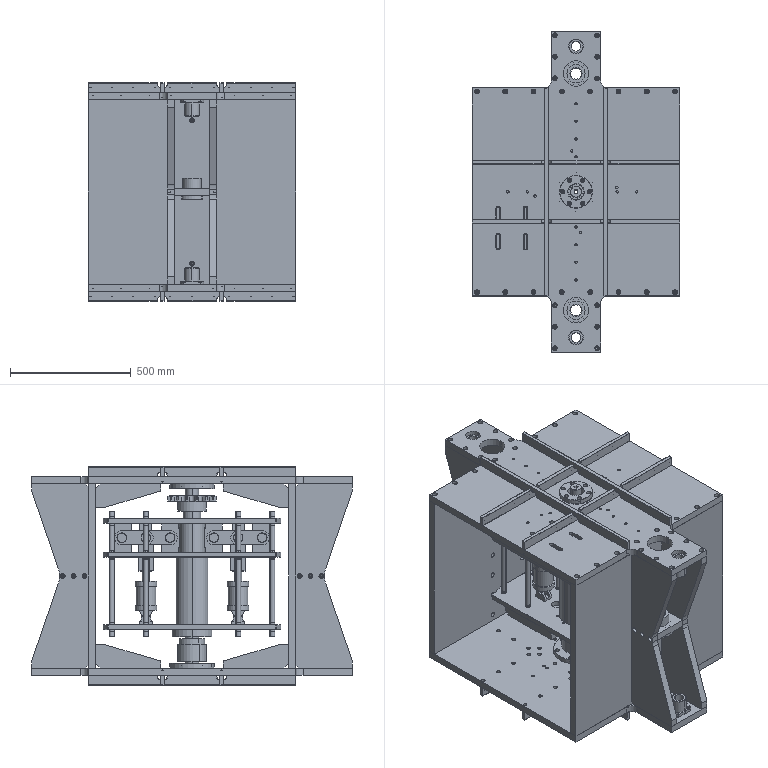Part | SolidWorks | 128 solids | 6123 faces | volume 136371359 mm3 | cylinder 2528 | plane 1981 | cone 1406 | sphere 144 | torus 64 | commonest cylinder face diameters 9 x346 10.2 x288 6.8 x248 13.5 x240 20 x232 15 x188